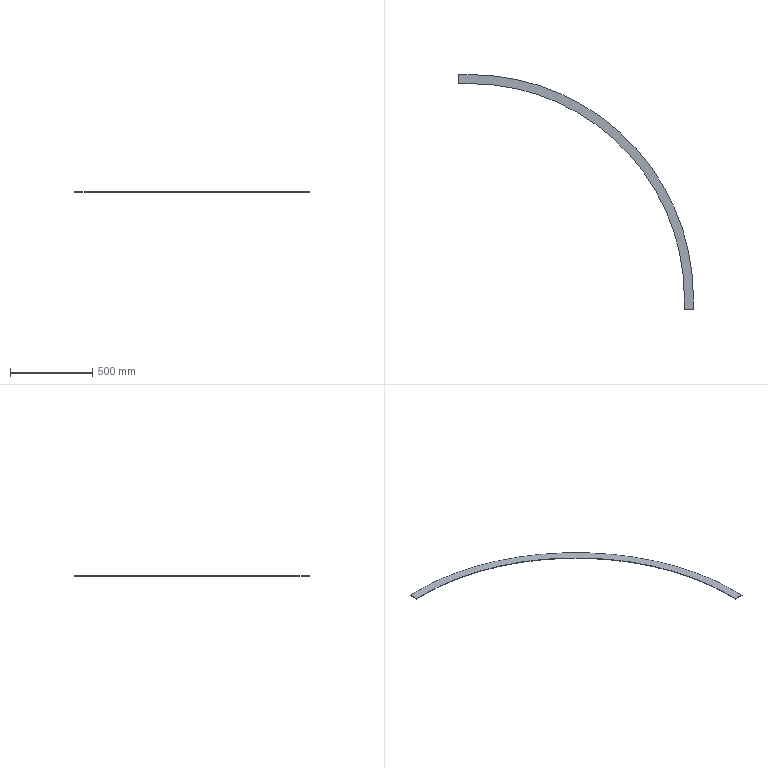Part | STEP file | covercurveroller-p2 | 1 solid | 10 faces | box 1428 x 1428 x 2.5 mm | volume 306725 mm3 | plane 8 | cylinder 2 | commonest cylinder face diameters 2607 x1 2717 x1
STEP:
#1=CARTESIAN_POINT('',(0.,0.,0.));
#2=DIRECTION('',(0.,0.,1.));
#3=DIRECTION('',(1.,0.,0.));
#4=AXIS2_PLACEMENT_3D('',#1,#2,#3);
#5=CARTESIAN_POINT('',(1479.114,-533.249,2.5));
#6=VERTEX_POINT('',#5);
#7=CARTESIAN_POINT('',(1479.114,-603.249,2.5));
#8=VERTEX_POINT('',#7);
#9=CARTESIAN_POINT('',(1479.114,-533.249,2.5));
#10=DIRECTION('',(0.,-1.,0.));
#11=VECTOR('',#10,1.);
#12=LINE('',#9,#11);
#13=CARTESIAN_POINT('',(1479.114,-533.249,0.));
#14=DIRECTION('',(1.,0.,0.));
#15=DIRECTION('',(0.,0.,-1.));
#16=AXIS2_PLACEMENT_3D('',#13,#14,#15);
#17=PLANE('',#16);
#18=CARTESIAN_POINT('',(-2.5,0.));
#19=DIRECTION('',(0.,-1.));
#20=VECTOR('',#19,1.);
#21=LINE('',#18,#20);
#22=(GEOMETRIC_REPRESENTATION_CONTEXT(2)PARAMETRIC_REPRESENTATION_CONTEXT()REPRESENTATION_CONTEXT('',''));
#23=DEFINITIONAL_REPRESENTATION('',(#21),#22);
#24=PCURVE('',#17,#23);
#25=CARTESIAN_POINT('',(934.281,280.419,2.5));
#26=DIRECTION('',(0.,0.,1.));
#27=DIRECTION('',(1.,0.,0.));
#28=AXIS2_PLACEMENT_3D('',#25,#26,#27);
#29=PLANE('',#28);
#30=CARTESIAN_POINT('',(544.833,-813.667));
#31=DIRECTION('',(0.,-1.));
#32=VECTOR('',#31,1.);
#33=LINE('',#30,#32);
#34=(GEOMETRIC_REPRESENTATION_CONTEXT(2)PARAMETRIC_REPRESENTATION_CONTEXT()REPRESENTATION_CONTEXT('',''));
#35=DEFINITIONAL_REPRESENTATION('',(#33),#34);
#36=PCURVE('',#29,#35);
#37=SURFACE_CURVE('',#12,(#24,#36),.PCURVE_S1.);
#38=EDGE_CURVE('',#6,#8,#37,.T.);
#39=ORIENTED_EDGE('',*,*,#38,.T.);
#40=CARTESIAN_POINT('',(1479.114,-603.249,0.));
#41=VERTEX_POINT('',#40);
#42=CARTESIAN_POINT('',(1479.114,-603.249,0.));
#43=DIRECTION('',(0.,0.,1.));
#44=VECTOR('',#43,1.);
#45=LINE('',#42,#44);
#46=CARTESIAN_POINT('',(0.,-70.));
#47=DIRECTION('',(-1.,0.));
#48=VECTOR('',#47,1.);
#49=LINE('',#46,#48);
#50=(GEOMETRIC_REPRESENTATION_CONTEXT(2)PARAMETRIC_REPRESENTATION_CONTEXT()REPRESENTATION_CONTEXT('',''));
#51=DEFINITIONAL_REPRESENTATION('',(#49),#50);
#52=PCURVE('',#17,#51);
#53=CARTESIAN_POINT('',(1479.114,-603.249,0.));
#54=DIRECTION('',(0.,-1.,0.));
#55=DIRECTION('',(0.,0.,-1.));
#56=AXIS2_PLACEMENT_3D('',#53,#54,#55);
#57=PLANE('',#56);
#58=CARTESIAN_POINT('',(0.,0.));
#59=DIRECTION('',(-1.,0.));
#60=VECTOR('',#59,1.);
#61=LINE('',#58,#60);
#62=(GEOMETRIC_REPRESENTATION_CONTEXT(2)PARAMETRIC_REPRESENTATION_CONTEXT()REPRESENTATION_CONTEXT('',''));
#63=DEFINITIONAL_REPRESENTATION('',(#61),#62);
#64=PCURVE('',#57,#63);
#65=SURFACE_CURVE('',#45,(#52,#64),.PCURVE_S1.);
#66=EDGE_CURVE('',#41,#8,#65,.T.);
#67=ORIENTED_EDGE('',*,*,#66,.F.);
#68=CARTESIAN_POINT('',(1479.114,-533.249,0.));
#69=VERTEX_POINT('',#68);
#70=CARTESIAN_POINT('',(1479.114,-533.249,0.));
#71=DIRECTION('',(0.,-1.,0.));
#72=VECTOR('',#71,1.);
#73=LINE('',#70,#72);
#74=CARTESIAN_POINT('',(0.,0.));
#75=DIRECTION('',(0.,-1.));
#76=VECTOR('',#75,1.);
#77=LINE('',#74,#76);
#78=(GEOMETRIC_REPRESENTATION_CONTEXT(2)PARAMETRIC_REPRESENTATION_CONTEXT()REPRESENTATION_CONTEXT('',''));
#79=DEFINITIONAL_REPRESENTATION('',(#77),#78);
#80=PCURVE('',#17,#79);
#81=CARTESIAN_POINT('',(934.281,280.419,0.));
#82=DIRECTION('',(0.,0.,1.));
#83=DIRECTION('',(1.,0.,0.));
#84=AXIS2_PLACEMENT_3D('',#81,#82,#83);
#85=PLANE('',#84);
#86=CARTESIAN_POINT('',(544.833,-813.667));
#87=DIRECTION('',(0.,-1.));
#88=VECTOR('',#87,1.);
#89=LINE('',#86,#88);
#90=(GEOMETRIC_REPRESENTATION_CONTEXT(2)PARAMETRIC_REPRESENTATION_CONTEXT()REPRESENTATION_CONTEXT('',''));
#91=DEFINITIONAL_REPRESENTATION('',(#89),#90);
#92=PCURVE('',#85,#91);
#93=SURFACE_CURVE('',#73,(#80,#92),.PCURVE_S1.);
#94=EDGE_CURVE('',#69,#41,#93,.T.);
#95=ORIENTED_EDGE('',*,*,#94,.F.);
#96=CARTESIAN_POINT('',(1479.114,-533.249,0.));
#97=DIRECTION('',(0.,0.,1.));
#98=VECTOR('',#97,1.);
#99=LINE('',#96,#98);
#100=CARTESIAN_POINT('',(0.,0.));
#101=DIRECTION('',(-1.,0.));
#102=VECTOR('',#101,1.);
#103=LINE('',#100,#102);
#104=(GEOMETRIC_REPRESENTATION_CONTEXT(2)PARAMETRIC_REPRESENTATION_CONTEXT()REPRESENTATION_CONTEXT('',''));
#105=DEFINITIONAL_REPRESENTATION('',(#103),#104);
#106=PCURVE('',#17,#105);
#107=CARTESIAN_POINT('',(120.614,-533.249,0.));
#108=DIRECTION('',(0.,0.,1.));
#109=DIRECTION('',(-1.,0.,0.));
#110=AXIS2_PLACEMENT_3D('',#107,#108,#109);
#111=CYLINDRICAL_SURFACE('',#110,1358.5);
#112=CARTESIAN_POINT('',(3.142,0.));
#113=DIRECTION('',(0.,1.));
#114=VECTOR('',#113,1.);
#115=LINE('',#112,#114);
#116=(GEOMETRIC_REPRESENTATION_CONTEXT(2)PARAMETRIC_REPRESENTATION_CONTEXT()REPRESENTATION_CONTEXT('',''));
#117=DEFINITIONAL_REPRESENTATION('',(#115),#116);
#118=PCURVE('',#111,#117);
#119=SURFACE_CURVE('',#99,(#106,#118),.PCURVE_S1.);
#120=EDGE_CURVE('',#69,#6,#119,.T.);
#121=ORIENTED_EDGE('',*,*,#120,.T.);
#122=EDGE_LOOP('',(#39,#67,#95,#121));
#123=FACE_BOUND('',#122,.T.);
#124=ADVANCED_FACE('',(#123),#17,.T.);
#125=CARTESIAN_POINT('',(1424.114,-603.249,2.5));
#126=VERTEX_POINT('',#125);
#127=CARTESIAN_POINT('',(1479.114,-603.249,2.5));
#128=DIRECTION('',(-1.,0.,0.));
#129=VECTOR('',#128,1.);
#130=LINE('',#127,#129);
#131=CARTESIAN_POINT('',(-2.5,0.));
#132=DIRECTION('',(0.,-1.));
#133=VECTOR('',#132,1.);
#134=LINE('',#131,#133);
#135=(GEOMETRIC_REPRESENTATION_CONTEXT(2)PARAMETRIC_REPRESENTATION_CONTEXT()REPRESENTATION_CONTEXT('',''));
#136=DEFINITIONAL_REPRESENTATION('',(#134),#135);
#137=PCURVE('',#57,#136);
#138=CARTESIAN_POINT('',(544.833,-883.667));
#139=DIRECTION('',(-1.,0.));
#140=VECTOR('',#139,1.);
#141=LINE('',#138,#140);
#142=(GEOMETRIC_REPRESENTATION_CONTEXT(2)PARAMETRIC_REPRESENTATION_CONTEXT()REPRESENTATION_CONTEXT('',''));
#143=DEFINITIONAL_REPRESENTATION('',(#141),#142);
#144=PCURVE('',#29,#143);
#145=SURFACE_CURVE('',#130,(#137,#144),.PCURVE_S1.);
#146=EDGE_CURVE('',#8,#126,#145,.T.);
#147=ORIENTED_EDGE('',*,*,#146,.T.);
#148=CARTESIAN_POINT('',(1424.114,-603.249,0.));
#149=VERTEX_POINT('',#148);
#150=CARTESIAN_POINT('',(1424.114,-603.249,0.));
#151=DIRECTION('',(0.,0.,1.));
#152=VECTOR('',#151,1.);
#153=LINE('',#150,#152);
#154=CARTESIAN_POINT('',(0.,-55.));
#155=DIRECTION('',(-1.,0.));
#156=VECTOR('',#155,1.);
#157=LINE('',#154,#156);
#158=(GEOMETRIC_REPRESENTATION_CONTEXT(2)PARAMETRIC_REPRESENTATION_CONTEXT()REPRESENTATION_CONTEXT('',''));
#159=DEFINITIONAL_REPRESENTATION('',(#157),#158);
#160=PCURVE('',#57,#159);
#161=CARTESIAN_POINT('',(1424.114,-603.249,0.));
#162=DIRECTION('',(-1.,0.,0.));
#163=DIRECTION('',(0.,0.,1.));
#164=AXIS2_PLACEMENT_3D('',#161,#162,#163);
#165=PLANE('',#164);
#166=CARTESIAN_POINT('',(0.,0.));
#167=DIRECTION('',(1.,0.));
#168=VECTOR('',#167,1.);
#169=LINE('',#166,#168);
#170=(GEOMETRIC_REPRESENTATION_CONTEXT(2)PARAMETRIC_REPRESENTATION_CONTEXT()REPRESENTATION_CONTEXT('',''));
#171=DEFINITIONAL_REPRESENTATION('',(#169),#170);
#172=PCURVE('',#165,#171);
#173=SURFACE_CURVE('',#153,(#160,#172),.PCURVE_S1.);
#174=EDGE_CURVE('',#149,#126,#173,.T.);
#175=ORIENTED_EDGE('',*,*,#174,.F.);
#176=CARTESIAN_POINT('',(1479.114,-603.249,0.));
#177=DIRECTION('',(-1.,0.,0.));
#178=VECTOR('',#177,1.);
#179=LINE('',#176,#178);
#180=CARTESIAN_POINT('',(0.,0.));
#181=DIRECTION('',(0.,-1.));
#182=VECTOR('',#181,1.);
#183=LINE('',#180,#182);
#184=(GEOMETRIC_REPRESENTATION_CONTEXT(2)PARAMETRIC_REPRESENTATION_CONTEXT()REPRESENTATION_CONTEXT('',''));
#185=DEFINITIONAL_REPRESENTATION('',(#183),#184);
#186=PCURVE('',#57,#185);
#187=CARTESIAN_POINT('',(544.833,-883.667));
#188=DIRECTION('',(-1.,0.));
#189=VECTOR('',#188,1.);
#190=LINE('',#187,#189);
#191=(GEOMETRIC_REPRESENTATION_CONTEXT(2)PARAMETRIC_REPRESENTATION_CONTEXT()REPRESENTATION_CONTEXT('',''));
#192=DEFINITIONAL_REPRESENTATION('',(#190),#191);
#193=PCURVE('',#85,#192);
#194=SURFACE_CURVE('',#179,(#186,#193),.PCURVE_S1.);
#195=EDGE_CURVE('',#41,#149,#194,.T.);
#196=ORIENTED_EDGE('',*,*,#195,.F.);
#197=ORIENTED_EDGE('',*,*,#66,.T.);
#198=EDGE_LOOP('',(#147,#175,#196,#197));
#199=FACE_BOUND('',#198,.T.);
#200=ADVANCED_FACE('',(#199),#57,.T.);
#201=CARTESIAN_POINT('',(1424.114,-533.249,2.5));
#202=VERTEX_POINT('',#201);
#203=CARTESIAN_POINT('',(1424.114,-603.249,2.5));
#204=DIRECTION('',(0.,1.,0.));
#205=VECTOR('',#204,1.);
#206=LINE('',#203,#205);
#207=CARTESIAN_POINT('',(2.5,0.));
#208=DIRECTION('',(0.,1.));
#209=VECTOR('',#208,1.);
#210=LINE('',#207,#209);
#211=(GEOMETRIC_REPRESENTATION_CONTEXT(2)PARAMETRIC_REPRESENTATION_CONTEXT()REPRESENTATION_CONTEXT('',''));
#212=DEFINITIONAL_REPRESENTATION('',(#210),#211);
#213=PCURVE('',#165,#212);
#214=CARTESIAN_POINT('',(489.833,-883.667));
#215=DIRECTION('',(0.,1.));
#216=VECTOR('',#215,1.);
#217=LINE('',#214,#216);
#218=(GEOMETRIC_REPRESENTATION_CONTEXT(2)PARAMETRIC_REPRESENTATION_CONTEXT()REPRESENTATION_CONTEXT('',''));
#219=DEFINITIONAL_REPRESENTATION('',(#217),#218);
#220=PCURVE('',#29,#219);
#221=SURFACE_CURVE('',#206,(#213,#220),.PCURVE_S1.);
#222=EDGE_CURVE('',#126,#202,#221,.T.);
#223=ORIENTED_EDGE('',*,*,#222,.T.);
#224=CARTESIAN_POINT('',(1424.114,-533.249,0.));
#225=VERTEX_POINT('',#224);
#226=CARTESIAN_POINT('',(1424.114,-533.249,0.));
#227=DIRECTION('',(0.,0.,1.));
#228=VECTOR('',#227,1.);
#229=LINE('',#226,#228);
#230=CARTESIAN_POINT('',(0.,70.));
#231=DIRECTION('',(1.,0.));
#232=VECTOR('',#231,1.);
#233=LINE('',#230,#232);
#234=(GEOMETRIC_REPRESENTATION_CONTEXT(2)PARAMETRIC_REPRESENTATION_CONTEXT()REPRESENTATION_CONTEXT('',''));
#235=DEFINITIONAL_REPRESENTATION('',(#233),#234);
#236=PCURVE('',#165,#235);
#237=CARTESIAN_POINT('',(120.614,-533.249,0.));
#238=DIRECTION('',(0.,0.,1.));
#239=DIRECTION('',(1.,0.,0.));
#240=AXIS2_PLACEMENT_3D('',#237,#238,#239);
#241=CYLINDRICAL_SURFACE('',#240,1303.5);
#242=CARTESIAN_POINT('',(0.,0.));
#243=DIRECTION('',(0.,1.));
#244=VECTOR('',#243,1.);
#245=LINE('',#242,#244);
#246=(GEOMETRIC_REPRESENTATION_CONTEXT(2)PARAMETRIC_REPRESENTATION_CONTEXT()REPRESENTATION_CONTEXT('',''));
#247=DEFINITIONAL_REPRESENTATION('',(#245),#246);
#248=PCURVE('',#241,#247);
#249=SURFACE_CURVE('',#229,(#236,#248),.PCURVE_S1.);
#250=EDGE_CURVE('',#225,#202,#249,.T.);
#251=ORIENTED_EDGE('',*,*,#250,.F.);
#252=CARTESIAN_POINT('',(1424.114,-603.249,0.));
#253=DIRECTION('',(0.,1.,0.));
#254=VECTOR('',#253,1.);
#255=LINE('',#252,#254);
#256=CARTESIAN_POINT('',(0.,0.));
#257=DIRECTION('',(0.,1.));
#258=VECTOR('',#257,1.);
#259=LINE('',#256,#258);
#260=(GEOMETRIC_REPRESENTATION_CONTEXT(2)PARAMETRIC_REPRESENTATION_CONTEXT()REPRESENTATION_CONTEXT('',''));
#261=DEFINITIONAL_REPRESENTATION('',(#259),#260);
#262=PCURVE('',#165,#261);
#263=CARTESIAN_POINT('',(489.833,-883.667));
#264=DIRECTION('',(0.,1.));
#265=VECTOR('',#264,1.);
#266=LINE('',#263,#265);
#267=(GEOMETRIC_REPRESENTATION_CONTEXT(2)PARAMETRIC_REPRESENTATION_CONTEXT()REPRESENTATION_CONTEXT('',''));
#268=DEFINITIONAL_REPRESENTATION('',(#266),#267);
#269=PCURVE('',#85,#268);
#270=SURFACE_CURVE('',#255,(#262,#269),.PCURVE_S1.);
#271=EDGE_CURVE('',#149,#225,#270,.T.);
#272=ORIENTED_EDGE('',*,*,#271,.F.);
#273=ORIENTED_EDGE('',*,*,#174,.T.);
#274=EDGE_LOOP('',(#223,#251,#272,#273));
#275=FACE_BOUND('',#274,.T.);
#276=ADVANCED_FACE('',(#275),#165,.T.);
#277=ORIENTED_EDGE('',*,*,#250,.F.);
#278=CARTESIAN_POINT('',(120.614,770.251,0.));
#279=VERTEX_POINT('',#278);
#280=CARTESIAN_POINT('',(120.614,-533.249,0.));
#281=DIRECTION('',(0.,0.,1.));
#282=DIRECTION('',(1.,0.,0.));
#283=AXIS2_PLACEMENT_3D('',#280,#281,#282);
#284=CIRCLE('',#283,1303.5);
#285=CARTESIAN_POINT('',(0.,0.));
#286=DIRECTION('',(1.,0.));
#287=VECTOR('',#286,1.);
#288=LINE('',#285,#287);
#289=(GEOMETRIC_REPRESENTATION_CONTEXT(2)PARAMETRIC_REPRESENTATION_CONTEXT()REPRESENTATION_CONTEXT('',''));
#290=DEFINITIONAL_REPRESENTATION('',(#288),#289);
#291=PCURVE('',#241,#290);
#292=CARTESIAN_POINT('',(-813.667,-813.667));
#293=DIRECTION('',(1.,0.));
#294=AXIS2_PLACEMENT_2D('',#292,#293);
#295=CIRCLE('',#294,1303.5);
#296=(GEOMETRIC_REPRESENTATION_CONTEXT(2)PARAMETRIC_REPRESENTATION_CONTEXT()REPRESENTATION_CONTEXT('',''));
#297=DEFINITIONAL_REPRESENTATION('',(#295),#296);
#298=PCURVE('',#85,#297);
#299=SURFACE_CURVE('',#284,(#291,#298),.PCURVE_S1.);
#300=EDGE_CURVE('',#225,#279,#299,.T.);
#301=ORIENTED_EDGE('',*,*,#300,.T.);
#302=CARTESIAN_POINT('',(120.614,770.251,2.5));
#303=VERTEX_POINT('',#302);
#304=CARTESIAN_POINT('',(120.614,770.251,0.));
#305=DIRECTION('',(0.,0.,1.));
#306=VECTOR('',#305,1.);
#307=LINE('',#304,#306);
#308=CARTESIAN_POINT('',(1.571,0.));
#309=DIRECTION('',(0.,1.));
#310=VECTOR('',#309,1.);
#311=LINE('',#308,#310);
#312=(GEOMETRIC_REPRESENTATION_CONTEXT(2)PARAMETRIC_REPRESENTATION_CONTEXT()REPRESENTATION_CONTEXT('',''));
#313=DEFINITIONAL_REPRESENTATION('',(#311),#312);
#314=PCURVE('',#241,#313);
#315=CARTESIAN_POINT('',(120.614,770.251,0.));
#316=DIRECTION('',(0.,-1.,0.));
#317=DIRECTION('',(0.,0.,-1.));
#318=AXIS2_PLACEMENT_3D('',#315,#316,#317);
#319=PLANE('',#318);
#320=CARTESIAN_POINT('',(0.,0.));
#321=DIRECTION('',(-1.,0.));
#322=VECTOR('',#321,1.);
#323=LINE('',#320,#322);
#324=(GEOMETRIC_REPRESENTATION_CONTEXT(2)PARAMETRIC_REPRESENTATION_CONTEXT()REPRESENTATION_CONTEXT('',''));
#325=DEFINITIONAL_REPRESENTATION('',(#323),#324);
#326=PCURVE('',#319,#325);
#327=SURFACE_CURVE('',#307,(#314,#326),.PCURVE_S1.);
#328=EDGE_CURVE('',#279,#303,#327,.T.);
#329=ORIENTED_EDGE('',*,*,#328,.T.);
#330=CARTESIAN_POINT('',(120.614,-533.249,2.5));
#331=DIRECTION('',(0.,0.,1.));
#332=DIRECTION('',(1.,0.,0.));
#333=AXIS2_PLACEMENT_3D('',#330,#331,#332);
#334=CIRCLE('',#333,1303.5);
#335=CARTESIAN_POINT('',(0.,2.5));
#336=DIRECTION('',(1.,0.));
#337=VECTOR('',#336,1.);
#338=LINE('',#335,#337);
#339=(GEOMETRIC_REPRESENTATION_CONTEXT(2)PARAMETRIC_REPRESENTATION_CONTEXT()REPRESENTATION_CONTEXT('',''));
#340=DEFINITIONAL_REPRESENTATION('',(#338),#339);
#341=PCURVE('',#241,#340);
#342=CARTESIAN_POINT('',(-813.667,-813.667));
#343=DIRECTION('',(1.,0.));
#344=AXIS2_PLACEMENT_2D('',#342,#343);
#345=CIRCLE('',#344,1303.5);
#346=(GEOMETRIC_REPRESENTATION_CONTEXT(2)PARAMETRIC_REPRESENTATION_CONTEXT()REPRESENTATION_CONTEXT('',''));
#347=DEFINITIONAL_REPRESENTATION('',(#345),#346);
#348=PCURVE('',#29,#347);
#349=SURFACE_CURVE('',#334,(#341,#348),.PCURVE_S1.);
#350=EDGE_CURVE('',#202,#303,#349,.T.);
#351=ORIENTED_EDGE('',*,*,#350,.F.);
#352=EDGE_LOOP('',(#277,#301,#329,#351));
#353=FACE_BOUND('',#352,.F.);
#354=ADVANCED_FACE('',(#353),#241,.F.);
#355=CARTESIAN_POINT('',(50.614,770.251,2.5));
#356=VERTEX_POINT('',#355);
#357=CARTESIAN_POINT('',(120.614,770.251,2.5));
#358=DIRECTION('',(-1.,0.,0.));
#359=VECTOR('',#358,1.);
#360=LINE('',#357,#359);
#361=CARTESIAN_POINT('',(-2.5,0.));
#362=DIRECTION('',(0.,-1.));
#363=VECTOR('',#362,1.);
#364=LINE('',#361,#363);
#365=(GEOMETRIC_REPRESENTATION_CONTEXT(2)PARAMETRIC_REPRESENTATION_CONTEXT()REPRESENTATION_CONTEXT('',''));
#366=DEFINITIONAL_REPRESENTATION('',(#364),#365);
#367=PCURVE('',#319,#366);
#368=CARTESIAN_POINT('',(-813.667,489.833));
#369=DIRECTION('',(-1.,0.));
#370=VECTOR('',#369,1.);
#371=LINE('',#368,#370);
#372=(GEOMETRIC_REPRESENTATION_CONTEXT(2)PARAMETRIC_REPRESENTATION_CONTEXT()REPRESENTATION_CONTEXT('',''));
#373=DEFINITIONAL_REPRESENTATION('',(#371),#372);
#374=PCURVE('',#29,#373);
#375=SURFACE_CURVE('',#360,(#367,#374),.PCURVE_S1.);
#376=EDGE_CURVE('',#303,#356,#375,.T.);
#377=ORIENTED_EDGE('',*,*,#376,.T.);
#378=CARTESIAN_POINT('',(50.614,770.251,0.));
#379=VERTEX_POINT('',#378);
#380=CARTESIAN_POINT('',(50.614,770.251,0.));
#381=DIRECTION('',(0.,0.,1.));
#382=VECTOR('',#381,1.);
#383=LINE('',#380,#382);
#384=CARTESIAN_POINT('',(0.,-70.));
#385=DIRECTION('',(-1.,0.));
#386=VECTOR('',#385,1.);
#387=LINE('',#384,#386);
#388=(GEOMETRIC_REPRESENTATION_CONTEXT(2)PARAMETRIC_REPRESENTATION_CONTEXT()REPRESENTATION_CONTEXT('',''));
#389=DEFINITIONAL_REPRESENTATION('',(#387),#388);
#390=PCURVE('',#319,#389);
#391=CARTESIAN_POINT('',(50.614,770.251,0.));
#392=DIRECTION('',(-1.,0.,0.));
#393=DIRECTION('',(0.,0.,1.));
#394=AXIS2_PLACEMENT_3D('',#391,#392,#393);
#395=PLANE('',#394);
#396=CARTESIAN_POINT('',(0.,0.));
#397=DIRECTION('',(1.,0.));
#398=VECTOR('',#397,1.);
#399=LINE('',#396,#398);
#400=(GEOMETRIC_REPRESENTATION_CONTEXT(2)PARAMETRIC_REPRESENTATION_CONTEXT()REPRESENTATION_CONTEXT('',''));
#401=DEFINITIONAL_REPRESENTATION('',(#399),#400);
#402=PCURVE('',#395,#401);
#403=SURFACE_CURVE('',#383,(#390,#402),.PCURVE_S1.);
#404=EDGE_CURVE('',#379,#356,#403,.T.);
#405=ORIENTED_EDGE('',*,*,#404,.F.);
#406=CARTESIAN_POINT('',(120.614,770.251,0.));
#407=DIRECTION('',(-1.,0.,0.));
#408=VECTOR('',#407,1.);
#409=LINE('',#406,#408);
#410=CARTESIAN_POINT('',(0.,0.));
#411=DIRECTION('',(0.,-1.));
#412=VECTOR('',#411,1.);
#413=LINE('',#410,#412);
#414=(GEOMETRIC_REPRESENTATION_CONTEXT(2)PARAMETRIC_REPRESENTATION_CONTEXT()REPRESENTATION_CONTEXT('',''));
#415=DEFINITIONAL_REPRESENTATION('',(#413),#414);
#416=PCURVE('',#319,#415);
#417=CARTESIAN_POINT('',(-813.667,489.833));
#418=DIRECTION('',(-1.,0.));
#419=VECTOR('',#418,1.);
#420=LINE('',#417,#419);
#421=(GEOMETRIC_REPRESENTATION_CONTEXT(2)PARAMETRIC_REPRESENTATION_CONTEXT()REPRESENTATION_CONTEXT('',''));
#422=DEFINITIONAL_REPRESENTATION('',(#420),#421);
#423=PCURVE('',#85,#422);
#424=SURFACE_CURVE('',#409,(#416,#423),.PCURVE_S1.);
#425=EDGE_CURVE('',#279,#379,#424,.T.);
#426=ORIENTED_EDGE('',*,*,#425,.F.);
#427=ORIENTED_EDGE('',*,*,#328,.T.);
#428=EDGE_LOOP('',(#377,#405,#426,#427));
#429=FACE_BOUND('',#428,.T.);
#430=ADVANCED_FACE('',(#429),#319,.T.);
#431=CARTESIAN_POINT('',(50.614,825.251,2.5));
#432=VERTEX_POINT('',#431);
#433=CARTESIAN_POINT('',(50.614,770.251,2.5));
#434=DIRECTION('',(0.,1.,0.));
#435=VECTOR('',#434,1.);
#436=LINE('',#433,#435);
#437=CARTESIAN_POINT('',(2.5,0.));
#438=DIRECTION('',(0.,1.));
#439=VECTOR('',#438,1.);
#440=LINE('',#437,#439);
#441=(GEOMETRIC_REPRESENTATION_CONTEXT(2)PARAMETRIC_REPRESENTATION_CONTEXT()REPRESENTATION_CONTEXT('',''));
#442=DEFINITIONAL_REPRESENTATION('',(#440),#441);
#443=PCURVE('',#395,#442);
#444=CARTESIAN_POINT('',(-883.667,489.833));
#445=DIRECTION('',(0.,1.));
#446=VECTOR('',#445,1.);
#447=LINE('',#444,#446);
#448=(GEOMETRIC_REPRESENTATION_CONTEXT(2)PARAMETRIC_REPRESENTATION_CONTEXT()REPRESENTATION_CONTEXT('',''));
#449=DEFINITIONAL_REPRESENTATION('',(#447),#448);
#450=PCURVE('',#29,#449);
#451=SURFACE_CURVE('',#436,(#443,#450),.PCURVE_S1.);
#452=EDGE_CURVE('',#356,#432,#451,.T.);
#453=ORIENTED_EDGE('',*,*,#452,.T.);
#454=CARTESIAN_POINT('',(50.614,825.251,0.));
#455=VERTEX_POINT('',#454);
#456=CARTESIAN_POINT('',(50.614,825.251,0.));
#457=DIRECTION('',(0.,0.,1.));
#458=VECTOR('',#457,1.);
#459=LINE('',#456,#458);
#460=CARTESIAN_POINT('',(0.,55.));
#461=DIRECTION('',(1.,0.));
#462=VECTOR('',#461,1.);
#463=LINE('',#460,#462);
#464=(GEOMETRIC_REPRESENTATION_CONTEXT(2)PARAMETRIC_REPRESENTATION_CONTEXT()REPRESENTATION_CONTEXT('',''));
#465=DEFINITIONAL_REPRESENTATION('',(#463),#464);
#466=PCURVE('',#395,#465);
#467=CARTESIAN_POINT('',(50.614,825.251,0.));
#468=DIRECTION('',(0.,1.,0.));
#469=DIRECTION('',(0.,0.,1.));
#470=AXIS2_PLACEMENT_3D('',#467,#468,#469);
#471=PLANE('',#470);
#472=CARTESIAN_POINT('',(0.,0.));
#473=DIRECTION('',(1.,0.));
#474=VECTOR('',#473,1.);
#475=LINE('',#472,#474);
#476=(GEOMETRIC_REPRESENTATION_CONTEXT(2)PARAMETRIC_REPRESENTATION_CONTEXT()REPRESENTATION_CONTEXT('',''));
#477=DEFINITIONAL_REPRESENTATION('',(#475),#476);
#478=PCURVE('',#471,#477);
#479=SURFACE_CURVE('',#459,(#466,#478),.PCURVE_S1.);
#480=EDGE_CURVE('',#455,#432,#479,.T.);
#481=ORIENTED_EDGE('',*,*,#480,.F.);
#482=CARTESIAN_POINT('',(50.614,770.251,0.));
#483=DIRECTION('',(0.,1.,0.));
#484=VECTOR('',#483,1.);
#485=LINE('',#482,#484);
#486=CARTESIAN_POINT('',(0.,0.));
#487=DIRECTION('',(0.,1.));
#488=VECTOR('',#487,1.);
#489=LINE('',#486,#488);
#490=(GEOMETRIC_REPRESENTATION_CONTEXT(2)PARAMETRIC_REPRESENTATION_CONTEXT()REPRESENTATION_CONTEXT('',''));
#491=DEFINITIONAL_REPRESENTATION('',(#489),#490);
#492=PCURVE('',#395,#491);
#493=CARTESIAN_POINT('',(-883.667,489.833));
#494=DIRECTION('',(0.,1.));
#495=VECTOR('',#494,1.);
#496=LINE('',#493,#495);
#497=(GEOMETRIC_REPRESENTATION_CONTEXT(2)PARAMETRIC_REPRESENTATION_CONTEXT()REPRESENTATION_CONTEXT('',''));
#498=DEFINITIONAL_REPRESENTATION('',(#496),#497);
#499=PCURVE('',#85,#498);
#500=SURFACE_CURVE('',#485,(#492,#499),.PCURVE_S1.);
#501=EDGE_CURVE('',#379,#455,#500,.T.);
#502=ORIENTED_EDGE('',*,*,#501,.F.);
#503=ORIENTED_EDGE('',*,*,#404,.T.);
#504=EDGE_LOOP('',(#453,#481,#502,#503));
#505=FACE_BOUND('',#504,.T.);
#506=ADVANCED_FACE('',(#505),#395,.T.);
#507=CARTESIAN_POINT('',(120.614,825.251,2.5));
#508=VERTEX_POINT('',#507);
#509=CARTESIAN_POINT('',(50.614,825.251,2.5));
#510=DIRECTION('',(1.,0.,0.));
#511=VECTOR('',#510,1.);
#512=LINE('',#509,#511);
#513=CARTESIAN_POINT('',(2.5,0.));
#514=DIRECTION('',(0.,1.));
#515=VECTOR('',#514,1.);
#516=LINE('',#513,#515);
#517=(GEOMETRIC_REPRESENTATION_CONTEXT(2)PARAMETRIC_REPRESENTATION_CONTEXT()REPRESENTATION_CONTEXT('',''));
#518=DEFINITIONAL_REPRESENTATION('',(#516),#517);
#519=PCURVE('',#471,#518);
#520=CARTESIAN_POINT('',(-883.667,544.833));
#521=DIRECTION('',(1.,0.));
#522=VECTOR('',#521,1.);
#523=LINE('',#520,#522);
#524=(GEOMETRIC_REPRESENTATION_CONTEXT(2)PARAMETRIC_REPRESENTATION_CONTEXT()REPRESENTATION_CONTEXT('',''));
#525=DEFINITIONAL_REPRESENTATION('',(#523),#524);
#526=PCURVE('',#29,#525);
#527=SURFACE_CURVE('',#512,(#519,#526),.PCURVE_S1.);
#528=EDGE_CURVE('',#432,#508,#527,.T.);
#529=ORIENTED_EDGE('',*,*,#528,.T.);
#530=CARTESIAN_POINT('',(120.614,825.251,0.));
#531=VERTEX_POINT('',#530);
#532=CARTESIAN_POINT('',(120.614,825.251,0.));
#533=DIRECTION('',(0.,0.,1.));
#534=VECTOR('',#533,1.);
#535=LINE('',#532,#534);
#536=CARTESIAN_POINT('',(0.,70.));
#537=DIRECTION('',(1.,0.));
#538=VECTOR('',#537,1.);
#539=LINE('',#536,#538);
#540=(GEOMETRIC_REPRESENTATION_CONTEXT(2)PARAMETRIC_REPRESENTATION_CONTEXT()REPRESENTATION_CONTEXT('',''));
#541=DEFINITIONAL_REPRESENTATION('',(#539),#540);
#542=PCURVE('',#471,#541);
#543=CARTESIAN_POINT('',(4.712,0.));
#544=DIRECTION('',(0.,1.));
#545=VECTOR('',#544,1.);
#546=LINE('',#543,#545);
#547=(GEOMETRIC_REPRESENTATION_CONTEXT(2)PARAMETRIC_REPRESENTATION_CONTEXT()REPRESENTATION_CONTEXT('',''));
#548=DEFINITIONAL_REPRESENTATION('',(#546),#547);
#549=PCURVE('',#111,#548);
#550=SURFACE_CURVE('',#535,(#542,#549),.PCURVE_S1.);
#551=EDGE_CURVE('',#531,#508,#550,.T.);
#552=ORIENTED_EDGE('',*,*,#551,.F.);
#553=CARTESIAN_POINT('',(50.614,825.251,0.));
#554=DIRECTION('',(1.,0.,0.));
#555=VECTOR('',#554,1.);
#556=LINE('',#553,#555);
#557=CARTESIAN_POINT('',(0.,0.));
#558=DIRECTION('',(0.,1.));
#559=VECTOR('',#558,1.);
#560=LINE('',#557,#559);
#561=(GEOMETRIC_REPRESENTATION_CONTEXT(2)PARAMETRIC_REPRESENTATION_CONTEXT()REPRESENTATION_CONTEXT('',''));
#562=DEFINITIONAL_REPRESENTATION('',(#560),#561);
#563=PCURVE('',#471,#562);
#564=CARTESIAN_POINT('',(-883.667,544.833));
#565=DIRECTION('',(1.,0.));
#566=VECTOR('',#565,1.);
#567=LINE('',#564,#566);
#568=(GEOMETRIC_REPRESENTATION_CONTEXT(2)PARAMETRIC_REPRESENTATION_CONTEXT()REPRESENTATION_CONTEXT('',''));
#569=DEFINITIONAL_REPRESENTATION('',(#567),#568);
#570=PCURVE('',#85,#569);
#571=SURFACE_CURVE('',#556,(#563,#570),.PCURVE_S1.);
#572=EDGE_CURVE('',#455,#531,#571,.T.);
#573=ORIENTED_EDGE('',*,*,#572,.F.);
#574=ORIENTED_EDGE('',*,*,#480,.T.);
#575=EDGE_LOOP('',(#529,#552,#573,#574));
#576=FACE_BOUND('',#575,.T.);
#577=ADVANCED_FACE('',(#576),#471,.T.);
#578=CARTESIAN_POINT('',(120.614,-533.249,2.5));
#579=DIRECTION('',(0.,0.,-1.));
#580=DIRECTION('',(-1.,0.,0.));
#581=AXIS2_PLACEMENT_3D('',#578,#579,#580);
#582=CIRCLE('',#581,1358.5);
#583=CARTESIAN_POINT('',(6.283,2.5));
#584=DIRECTION('',(-1.,0.));
#585=VECTOR('',#584,1.);
#586=LINE('',#583,#585);
#587=(GEOMETRIC_REPRESENTATION_CONTEXT(2)PARAMETRIC_REPRESENTATION_CONTEXT()REPRESENTATION_CONTEXT('',''));
#588=DEFINITIONAL_REPRESENTATION('',(#586),#587);
#589=PCURVE('',#111,#588);
#590=CARTESIAN_POINT('',(-2172.167,-813.667));
#591=CARTESIAN_POINT('',(-2172.167,1539.324));
#592=CARTESIAN_POINT('',(-134.417,362.828));
#593=CARTESIAN_POINT('',(1903.333,-813.667));
#594=CARTESIAN_POINT('',(-134.417,-1990.163));
#595=CARTESIAN_POINT('',(-2172.167,-3166.658));
#596=CARTESIAN_POINT('',(-2172.167,-813.667));
#597=(BOUNDED_CURVE()B_SPLINE_CURVE(2,(#590,#591,#592,#593,#594,#595,#596),.UNSPECIFIED.,.T.,.F.)B_SPLINE_CURVE_WITH_KNOTS((1,2,2,2,2,1),(-2.094,0.,2.094,4.189,6.283,8.378),.UNSPECIFIED.)CURVE()GEOMETRIC_REPRESENTATION_ITEM()RATIONAL_B_SPLINE_CURVE((1.,0.5,1.,0.5,1.,0.5,1.))REPRESENTATION_ITEM(''));
#598=(GEOMETRIC_REPRESENTATION_CONTEXT(2)PARAMETRIC_REPRESENTATION_CONTEXT()REPRESENTATION_CONTEXT('',''));
#599=DEFINITIONAL_REPRESENTATION('',(#597),#598);
#600=PCURVE('',#29,#599);
#601=SURFACE_CURVE('',#582,(#589,#600),.PCURVE_S1.);
#602=EDGE_CURVE('',#508,#6,#601,.T.);
#603=ORIENTED_EDGE('',*,*,#602,.T.);
#604=ORIENTED_EDGE('',*,*,#120,.F.);
#605=CARTESIAN_POINT('',(120.614,-533.249,0.));
#606=DIRECTION('',(0.,0.,-1.));
#607=DIRECTION('',(-1.,0.,0.));
#608=AXIS2_PLACEMENT_3D('',#605,#606,#607);
#609=CIRCLE('',#608,1358.5);
#610=CARTESIAN_POINT('',(6.283,0.));
#611=DIRECTION('',(-1.,0.));
#612=VECTOR('',#611,1.);
#613=LINE('',#610,#612);
#614=(GEOMETRIC_REPRESENTATION_CONTEXT(2)PARAMETRIC_REPRESENTATION_CONTEXT()REPRESENTATION_CONTEXT('',''));
#615=DEFINITIONAL_REPRESENTATION('',(#613),#614);
#616=PCURVE('',#111,#615);
#617=CARTESIAN_POINT('',(-2172.167,-813.667));
#618=CARTESIAN_POINT('',(-2172.167,1539.324));
#619=CARTESIAN_POINT('',(-134.417,362.828));
#620=CARTESIAN_POINT('',(1903.333,-813.667));
#621=CARTESIAN_POINT('',(-134.417,-1990.163));
#622=CARTESIAN_POINT('',(-2172.167,-3166.658));
#623=CARTESIAN_POINT('',(-2172.167,-813.667));
#624=(BOUNDED_CURVE()B_SPLINE_CURVE(2,(#617,#618,#619,#620,#621,#622,#623),.UNSPECIFIED.,.T.,.F.)B_SPLINE_CURVE_WITH_KNOTS((1,2,2,2,2,1),(-2.094,0.,2.094,4.189,6.283,8.378),.UNSPECIFIED.)CURVE()GEOMETRIC_REPRESENTATION_ITEM()RATIONAL_B_SPLINE_CURVE((1.,0.5,1.,0.5,1.,0.5,1.))REPRESENTATION_ITEM(''));
#625=(GEOMETRIC_REPRESENTATION_CONTEXT(2)PARAMETRIC_REPRESENTATION_CONTEXT()REPRESENTATION_CONTEXT('',''));
#626=DEFINITIONAL_REPRESENTATION('',(#624),#625);
#627=PCURVE('',#85,#626);
#628=SURFACE_CURVE('',#609,(#616,#627),.PCURVE_S1.);
#629=EDGE_CURVE('',#531,#69,#628,.T.);
#630=ORIENTED_EDGE('',*,*,#629,.F.);
#631=ORIENTED_EDGE('',*,*,#551,.T.);
#632=EDGE_LOOP('',(#603,#604,#630,#631));
#633=FACE_BOUND('',#632,.T.);
#634=ADVANCED_FACE('',(#633),#111,.T.);
#635=ORIENTED_EDGE('',*,*,#38,.F.);
#636=ORIENTED_EDGE('',*,*,#602,.F.);
#637=ORIENTED_EDGE('',*,*,#528,.F.);
#638=ORIENTED_EDGE('',*,*,#452,.F.);
#639=ORIENTED_EDGE('',*,*,#376,.F.);
#640=ORIENTED_EDGE('',*,*,#350,.F.);
#641=ORIENTED_EDGE('',*,*,#222,.F.);
#642=ORIENTED_EDGE('',*,*,#146,.F.);
#643=EDGE_LOOP('',(#635,#636,#637,#638,#639,#640,#641,#642));
#644=FACE_BOUND('',#643,.T.);
#645=ADVANCED_FACE('',(#644),#29,.T.);
#646=ORIENTED_EDGE('',*,*,#629,.T.);
#647=ORIENTED_EDGE('',*,*,#94,.T.);
#648=ORIENTED_EDGE('',*,*,#195,.T.);
#649=ORIENTED_EDGE('',*,*,#271,.T.);
#650=ORIENTED_EDGE('',*,*,#300,.T.);
#651=ORIENTED_EDGE('',*,*,#425,.T.);
#652=ORIENTED_EDGE('',*,*,#501,.T.);
#653=ORIENTED_EDGE('',*,*,#572,.T.);
#654=EDGE_LOOP('',(#646,#647,#648,#649,#650,#651,#652,#653));
#655=FACE_BOUND('',#654,.T.);
#656=ADVANCED_FACE('',(#655),#85,.F.);
#657=CLOSED_SHELL('',(#124,#200,#276,#354,#430,#506,#577,#634,#645,#656));
#658=MANIFOLD_SOLID_BREP('',#657);
#659=(LENGTH_UNIT()NAMED_UNIT(*)SI_UNIT(.MILLI.,.METRE.));
#660=UNCERTAINTY_MEASURE_WITH_UNIT(LENGTH_MEASURE(0.0000001),#659,'','');
#661=(NAMED_UNIT(*)PLANE_ANGLE_UNIT()SI_UNIT($,.RADIAN.));
#662=(NAMED_UNIT(*)SI_UNIT($,.STERADIAN.)SOLID_ANGLE_UNIT());
#663=(GEOMETRIC_REPRESENTATION_CONTEXT(3)GLOBAL_UNCERTAINTY_ASSIGNED_CONTEXT((#660))GLOBAL_UNIT_ASSIGNED_CONTEXT((#659,#661,#662))REPRESENTATION_CONTEXT('',''));
#664=ADVANCED_BREP_SHAPE_REPRESENTATION('',(#4,#658),#663);